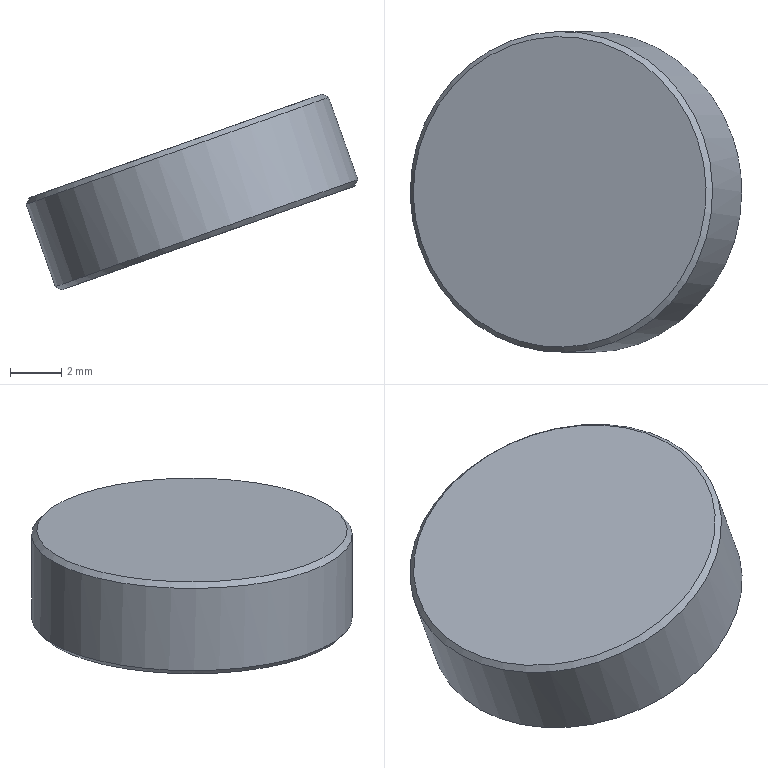Part | STEP file | ELECTRICAL-MICRO-SWITCH3_id6_x_t | 1 solid | 5 faces | box 12.918 x 12.5 x 7.621 mm | volume 464.776 mm3 | plane 2 | cone 2 | cylinder 1 | commonest cylinder face diameters 12.5 x1
STEP:
#1=CARTESIAN_POINT('',(54.838,-181.52,-33.499));
#2=VERTEX_POINT('',#1);
#3=CARTESIAN_POINT('',(60.214,-179.5,-31.595));
#4=DIRECTION('',(0.3338,0.,-0.9426));
#5=DIRECTION('',(-0.8886,-0.3338,-0.3147));
#6=AXIS2_PLACEMENT_3D('',#3,#4,#5);
#7=CIRCLE('',#6,6.05);
#8=EDGE_CURVE('',#2,#2,#7,.T.);
#9=ORIENTED_EDGE('',*,*,#8,.F.);
#10=EDGE_LOOP('',(#9));
#11=FACE_OUTER_BOUND('',#10,.T.);
#12=CARTESIAN_POINT('',(60.214,-80.713,-31.595));
#13=DIRECTION('',(-0.3338,0.,0.9426));
#14=DIRECTION('',(0.8886,0.3338,0.3147));
#15=AXIS2_PLACEMENT_3D('',#12,#13,#14);
#16=PLANE('',#15);
#17=ADVANCED_FACE('',(#11),#16,.T.);
#18=CARTESIAN_POINT('',(65.834,-177.414,-29.817));
#19=VERTEX_POINT('',#18);
#20=CARTESIAN_POINT('',(60.28,-179.5,-31.783));
#21=DIRECTION('',(0.3338,0.,-0.9426));
#22=DIRECTION('',(0.8886,0.3338,0.3147));
#23=AXIS2_PLACEMENT_3D('',#20,#21,#22);
#24=CIRCLE('',#23,6.25);
#25=EDGE_CURVE('',#19,#19,#24,.T.);
#26=ORIENTED_EDGE('',*,*,#25,.F.);
#27=EDGE_LOOP('',(#26));
#28=FACE_BOUND('',#27,.T.);
#29=ORIENTED_EDGE('',*,*,#8,.T.);
#30=EDGE_LOOP('',(#29));
#31=FACE_BOUND('',#30,.T.);
#32=CARTESIAN_POINT('',(60.28,-179.5,-31.783));
#33=DIRECTION('',(0.3338,0.,-0.9426));
#34=DIRECTION('',(-0.8886,-0.3338,-0.3147));
#35=AXIS2_PLACEMENT_3D('',#32,#33,#34);
#36=CONICAL_SURFACE('',#35,6.25,45.);
#37=ADVANCED_FACE('',(#28,#31),#36,.T.);
#38=ORIENTED_EDGE('',*,*,#25,.T.);
#39=EDGE_LOOP('',(#38));
#40=FACE_BOUND('',#39,.T.);
#41=CARTESIAN_POINT('',(67.307,-179.5,-32.902));
#42=VERTEX_POINT('',#41);
#43=CARTESIAN_POINT('',(61.415,-179.5,-34.988));
#44=DIRECTION('',(0.3338,0.,-0.9426));
#45=DIRECTION('',(0.9426,0.,0.3338));
#46=AXIS2_PLACEMENT_3D('',#43,#44,#45);
#47=CIRCLE('',#46,6.25);
#48=EDGE_CURVE('',#42,#42,#47,.T.);
#49=ORIENTED_EDGE('',*,*,#48,.F.);
#50=EDGE_LOOP('',(#49));
#51=FACE_BOUND('',#50,.T.);
#52=CARTESIAN_POINT('',(61.482,-179.5,-35.177));
#53=DIRECTION('',(-0.3338,0.,0.9426));
#54=DIRECTION('',(0.8886,0.3338,0.3147));
#55=AXIS2_PLACEMENT_3D('',#52,#53,#54);
#56=CYLINDRICAL_SURFACE('',#55,6.25);
#57=ADVANCED_FACE('',(#40,#51),#56,.T.);
#58=ORIENTED_EDGE('',*,*,#48,.T.);
#59=EDGE_LOOP('',(#58));
#60=FACE_BOUND('',#59,.T.);
#61=CARTESIAN_POINT('',(66.858,-177.48,-33.273));
#62=VERTEX_POINT('',#61);
#63=CARTESIAN_POINT('',(61.482,-179.5,-35.177));
#64=DIRECTION('',(-0.3338,0.,0.9426));
#65=DIRECTION('',(0.8886,0.3338,0.3147));
#66=AXIS2_PLACEMENT_3D('',#63,#64,#65);
#67=CIRCLE('',#66,6.05);
#68=EDGE_CURVE('',#62,#62,#67,.T.);
#69=ORIENTED_EDGE('',*,*,#68,.T.);
#70=EDGE_LOOP('',(#69));
#71=FACE_BOUND('',#70,.T.);
#72=CARTESIAN_POINT('',(61.415,-179.5,-34.988));
#73=DIRECTION('',(-0.3338,0.,0.9426));
#74=DIRECTION('',(0.8886,0.3338,0.3147));
#75=AXIS2_PLACEMENT_3D('',#72,#73,#74);
#76=CONICAL_SURFACE('',#75,6.25,45.);
#77=ADVANCED_FACE('',(#60,#71),#76,.T.);
#78=ORIENTED_EDGE('',*,*,#68,.F.);
#79=EDGE_LOOP('',(#78));
#80=FACE_OUTER_BOUND('',#79,.T.);
#81=CARTESIAN_POINT('',(61.482,-80.713,-35.177));
#82=DIRECTION('',(-0.3338,0.,0.9426));
#83=DIRECTION('',(0.8886,0.3338,0.3147));
#84=AXIS2_PLACEMENT_3D('',#81,#82,#83);
#85=PLANE('',#84);
#86=ADVANCED_FACE('',(#80),#85,.F.);
#87=CLOSED_SHELL('',(#17,#37,#57,#77,#86));
#88=MANIFOLD_SOLID_BREP('',#87);
#89=(LENGTH_UNIT()NAMED_UNIT(*)SI_UNIT(.MILLI.,.METRE.));
#90=UNCERTAINTY_MEASURE_WITH_UNIT(LENGTH_MEASURE(0.00002),#89,'','');
#91=(NAMED_UNIT(*)PLANE_ANGLE_UNIT()SI_UNIT($,.RADIAN.));
#92=PLANE_ANGLE_MEASURE_WITH_UNIT(PLANE_ANGLE_MEASURE(0.01745),#91);
#93=DIMENSIONAL_EXPONENTS(0.,0.,0.,0.,0.,0.,0.);
#94=(CONVERSION_BASED_UNIT('DEGREE',#92)NAMED_UNIT(#93)PLANE_ANGLE_UNIT());
#95=(NAMED_UNIT(*)SI_UNIT($,.STERADIAN.)SOLID_ANGLE_UNIT());
#96=(GEOMETRIC_REPRESENTATION_CONTEXT(3)GLOBAL_UNCERTAINTY_ASSIGNED_CONTEXT((#90))GLOBAL_UNIT_ASSIGNED_CONTEXT((#89,#94,#95))REPRESENTATION_CONTEXT('',''));
#97=ADVANCED_BREP_SHAPE_REPRESENTATION('',(#88),#96);